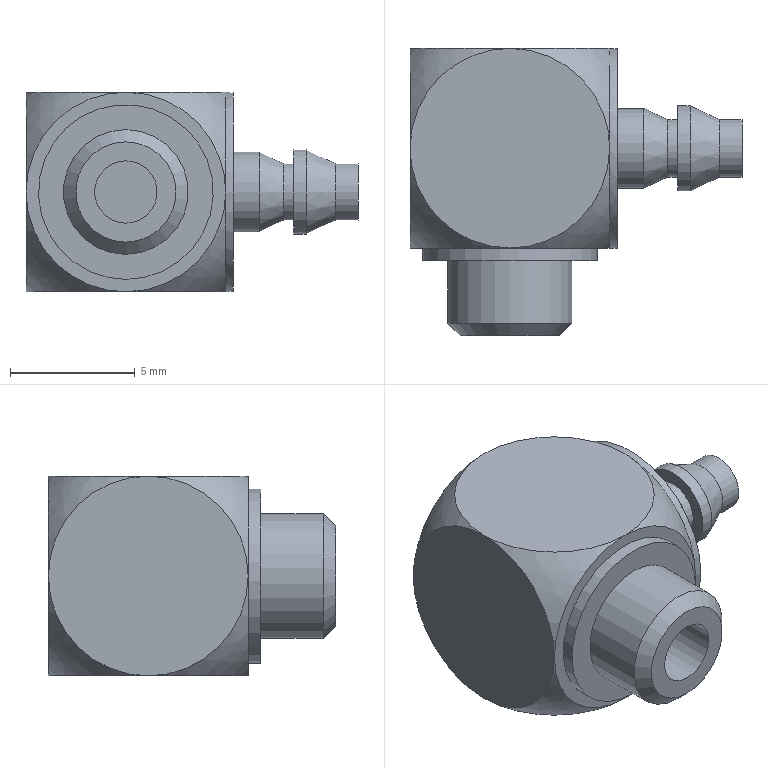Part | NX | 1 solid | 37 faces | box 13.3 x 11.5 x 8 mm | volume 560.169 mm3 | plane 15 | cylinder 11 | spline 8 | cone 3 | commonest cylinder face diameters 7 x3 2.3 x2 1.8 x1 2.5 x1 3.2 x1 3.4 x1
STEP:
#1=CARTESIAN_POINT('',(-4.,7.5,4.));
#2=VERTEX_POINT('',#1);
#3=CARTESIAN_POINT('',(0.,11.5,4.));
#4=VERTEX_POINT('',#3);
#5=CARTESIAN_POINT('',(-4.,7.5,4.));
#6=CARTESIAN_POINT('',(-4.,8.556,4.));
#7=CARTESIAN_POINT('',(-3.131,10.627,4.));
#8=CARTESIAN_POINT('',(-1.056,11.5,4.));
#9=CARTESIAN_POINT('',(0.,11.5,4.));
#10=B_SPLINE_CURVE_WITH_KNOTS('',3,(#5,#6,#7,#8,#9),.UNSPECIFIED.,.F.,.F.,(4,1,4),(0.,0.003124,0.006249),.UNSPECIFIED.);
#11=EDGE_CURVE('',#2,#4,#10,.T.);
#12=ORIENTED_EDGE('',*,*,#11,.F.);
#13=CARTESIAN_POINT('',(0.,3.5,4.));
#14=VERTEX_POINT('',#13);
#15=CARTESIAN_POINT('',(0.,3.5,4.));
#16=CARTESIAN_POINT('',(-1.056,3.5,4.));
#17=CARTESIAN_POINT('',(-3.127,4.369,4.));
#18=CARTESIAN_POINT('',(-4.,6.444,4.));
#19=CARTESIAN_POINT('',(-4.,7.5,4.));
#20=B_SPLINE_CURVE_WITH_KNOTS('',3,(#15,#16,#17,#18,#19),.UNSPECIFIED.,.F.,.F.,(4,1,4),(0.,0.003124,0.006249),.UNSPECIFIED.);
#21=EDGE_CURVE('',#14,#2,#20,.T.);
#22=ORIENTED_EDGE('',*,*,#21,.F.);
#23=CARTESIAN_POINT('',(4.,7.5,4.));
#24=VERTEX_POINT('',#23);
#25=CARTESIAN_POINT('',(4.,7.5,4.));
#26=CARTESIAN_POINT('',(4.,6.444,4.));
#27=CARTESIAN_POINT('',(3.131,4.373,4.));
#28=CARTESIAN_POINT('',(1.056,3.5,4.));
#29=CARTESIAN_POINT('',(0.,3.5,4.));
#30=B_SPLINE_CURVE_WITH_KNOTS('',3,(#25,#26,#27,#28,#29),.UNSPECIFIED.,.F.,.F.,(4,1,4),(0.,0.003124,0.006249),.UNSPECIFIED.);
#31=EDGE_CURVE('',#24,#14,#30,.T.);
#32=ORIENTED_EDGE('',*,*,#31,.F.);
#33=CARTESIAN_POINT('',(0.,11.5,4.));
#34=CARTESIAN_POINT('',(1.056,11.5,4.));
#35=CARTESIAN_POINT('',(3.127,10.631,4.));
#36=CARTESIAN_POINT('',(4.,8.556,4.));
#37=CARTESIAN_POINT('',(4.,7.5,4.));
#38=B_SPLINE_CURVE_WITH_KNOTS('',3,(#33,#34,#35,#36,#37),.UNSPECIFIED.,.F.,.F.,(4,1,4),(0.,0.003124,0.006249),.UNSPECIFIED.);
#39=EDGE_CURVE('',#4,#24,#38,.T.);
#40=ORIENTED_EDGE('',*,*,#39,.F.);
#41=EDGE_LOOP('',(#12,#22,#32,#40));
#42=FACE_BOUND('',#41,.T.);
#43=CARTESIAN_POINT('',(-4.,3.5,4.));
#44=DIRECTION('',(0.,0.,-1.));
#45=DIRECTION('',(-1.,0.,0.));
#46=AXIS2_PLACEMENT_3D('',#43,#44,#45);
#47=PLANE('',#46);
#48=ADVANCED_FACE('',(#42),#47,.F.);
#49=CARTESIAN_POINT('',(4.,11.5,0.));
#50=VERTEX_POINT('',#49);
#51=CARTESIAN_POINT('',(4.,11.5,0.));
#52=CARTESIAN_POINT('',(4.,11.5,1.056));
#53=CARTESIAN_POINT('',(3.131,11.5,3.127));
#54=CARTESIAN_POINT('',(1.056,11.5,4.));
#55=CARTESIAN_POINT('',(0.,11.5,4.));
#56=B_SPLINE_CURVE_WITH_KNOTS('',3,(#51,#52,#53,#54,#55),.UNSPECIFIED.,.F.,.F.,(4,1,4),(0.,0.003124,0.006249),.UNSPECIFIED.);
#57=EDGE_CURVE('',#50,#4,#56,.T.);
#58=ORIENTED_EDGE('',*,*,#57,.T.);
#59=ORIENTED_EDGE('',*,*,#39,.T.);
#60=CARTESIAN_POINT('',(4.,7.5,0.));
#61=DIRECTION('',(1.,0.,0.));
#62=DIRECTION('',(0.,1.,0.));
#63=AXIS2_PLACEMENT_3D('',#60,#61,#62);
#64=CIRCLE('',#63,4.);
#65=EDGE_CURVE('',#24,#50,#64,.F.);
#66=ORIENTED_EDGE('',*,*,#65,.T.);
#67=EDGE_LOOP('',(#58,#59,#66));
#68=FACE_BOUND('',#67,.T.);
#69=CARTESIAN_POINT('',(4.,11.5,0.));
#70=CARTESIAN_POINT('',(4.,11.5,2.361));
#71=CARTESIAN_POINT('',(4.,9.823,4.022));
#72=CARTESIAN_POINT('',(4.,7.462,4.));
#73=CARTESIAN_POINT('',(2.947,12.553,0.));
#74=CARTESIAN_POINT('',(2.947,12.553,2.982));
#75=CARTESIAN_POINT('',(2.947,10.435,5.081));
#76=CARTESIAN_POINT('',(2.947,7.452,5.053));
#77=CARTESIAN_POINT('',(1.463,13.164,0.));
#78=CARTESIAN_POINT('',(1.463,13.164,3.343));
#79=CARTESIAN_POINT('',(1.463,10.789,5.695));
#80=CARTESIAN_POINT('',(1.463,7.447,5.664));
#81=CARTESIAN_POINT('',(-0.02666,13.157,0.));
#82=CARTESIAN_POINT('',(-0.02666,13.157,3.338));
#83=CARTESIAN_POINT('',(-0.02666,10.785,5.688));
#84=CARTESIAN_POINT('',(-0.02666,7.447,5.657));
#85=(BOUNDED_SURFACE()B_SPLINE_SURFACE(3,3,((#69,#70,#71,#72),(#73,#74,#75,#76),(#77,#78,#79,#80),(#81,#82,#83,#84)),.SURF_OF_REVOLUTION.,.F.,.F.,.F.)B_SPLINE_SURFACE_WITH_KNOTS((4,4),(4,4),(0.7854,1.576),(0.,1.),.PIECEWISE_BEZIER_KNOTS.)GEOMETRIC_REPRESENTATION_ITEM()RATIONAL_B_SPLINE_SURFACE(((1.,0.8025,0.8025,1.),(1.,0.8025,0.8025,1.),(1.,0.8025,0.8025,1.),(1.,0.8025,0.8025,1.)))REPRESENTATION_ITEM('')SURFACE());
#86=ADVANCED_FACE('',(#68),#85,.T.);
#87=ORIENTED_EDGE('',*,*,#11,.T.);
#88=CARTESIAN_POINT('',(-4.,11.5,0.));
#89=VERTEX_POINT('',#88);
#90=CARTESIAN_POINT('',(0.,11.5,4.));
#91=CARTESIAN_POINT('',(-1.056,11.5,4.));
#92=CARTESIAN_POINT('',(-3.127,11.5,3.131));
#93=CARTESIAN_POINT('',(-4.,11.5,1.056));
#94=CARTESIAN_POINT('',(-4.,11.5,0.));
#95=B_SPLINE_CURVE_WITH_KNOTS('',3,(#90,#91,#92,#93,#94),.UNSPECIFIED.,.F.,.F.,(4,1,4),(0.,0.003124,0.006249),.UNSPECIFIED.);
#96=EDGE_CURVE('',#4,#89,#95,.T.);
#97=ORIENTED_EDGE('',*,*,#96,.T.);
#98=CARTESIAN_POINT('',(-4.,7.5,0.));
#99=DIRECTION('',(1.,0.,0.));
#100=DIRECTION('',(0.,0.,-1.));
#101=AXIS2_PLACEMENT_3D('',#98,#99,#100);
#102=CIRCLE('',#101,4.);
#103=EDGE_CURVE('',#89,#2,#102,.T.);
#104=ORIENTED_EDGE('',*,*,#103,.T.);
#105=EDGE_LOOP('',(#87,#97,#104));
#106=FACE_BOUND('',#105,.T.);
#107=CARTESIAN_POINT('',(0.02666,13.157,0.));
#108=CARTESIAN_POINT('',(0.02666,13.157,3.338));
#109=CARTESIAN_POINT('',(0.02666,10.785,5.688));
#110=CARTESIAN_POINT('',(0.02666,7.447,5.657));
#111=CARTESIAN_POINT('',(-1.463,13.164,0.));
#112=CARTESIAN_POINT('',(-1.463,13.164,3.343));
#113=CARTESIAN_POINT('',(-1.463,10.789,5.695));
#114=CARTESIAN_POINT('',(-1.463,7.447,5.664));
#115=CARTESIAN_POINT('',(-2.947,12.553,0.));
#116=CARTESIAN_POINT('',(-2.947,12.553,2.982));
#117=CARTESIAN_POINT('',(-2.947,10.435,5.081));
#118=CARTESIAN_POINT('',(-2.947,7.452,5.053));
#119=CARTESIAN_POINT('',(-4.,11.5,0.));
#120=CARTESIAN_POINT('',(-4.,11.5,2.361));
#121=CARTESIAN_POINT('',(-4.,9.823,4.022));
#122=CARTESIAN_POINT('',(-4.,7.462,4.));
#123=(BOUNDED_SURFACE()B_SPLINE_SURFACE(3,3,((#107,#108,#109,#110),(#111,#112,#113,#114),(#115,#116,#117,#118),(#119,#120,#121,#122)),.SURF_OF_REVOLUTION.,.F.,.F.,.F.)B_SPLINE_SURFACE_WITH_KNOTS((4,4),(4,4),(1.566,2.356),(0.,1.),.PIECEWISE_BEZIER_KNOTS.)GEOMETRIC_REPRESENTATION_ITEM()RATIONAL_B_SPLINE_SURFACE(((1.,0.8025,0.8025,1.),(1.,0.8025,0.8025,1.),(1.,0.8025,0.8025,1.),(1.,0.8025,0.8025,1.)))REPRESENTATION_ITEM('')SURFACE());
#124=ADVANCED_FACE('',(#106),#123,.T.);
#125=CARTESIAN_POINT('',(-4.,3.5,0.));
#126=VERTEX_POINT('',#125);
#127=CARTESIAN_POINT('',(-4.,3.5,0.));
#128=CARTESIAN_POINT('',(-4.,3.5,1.056));
#129=CARTESIAN_POINT('',(-3.131,3.5,3.127));
#130=CARTESIAN_POINT('',(-1.056,3.5,4.));
#131=CARTESIAN_POINT('',(0.,3.5,4.));
#132=B_SPLINE_CURVE_WITH_KNOTS('',3,(#127,#128,#129,#130,#131),.UNSPECIFIED.,.F.,.F.,(4,1,4),(0.,0.003124,0.006249),.UNSPECIFIED.);
#133=EDGE_CURVE('',#126,#14,#132,.T.);
#134=ORIENTED_EDGE('',*,*,#133,.T.);
#135=ORIENTED_EDGE('',*,*,#21,.T.);
#136=CARTESIAN_POINT('',(-4.,7.5,0.));
#137=DIRECTION('',(1.,0.,0.));
#138=DIRECTION('',(0.,0.,-1.));
#139=AXIS2_PLACEMENT_3D('',#136,#137,#138);
#140=CIRCLE('',#139,4.);
#141=EDGE_CURVE('',#2,#126,#140,.T.);
#142=ORIENTED_EDGE('',*,*,#141,.T.);
#143=EDGE_LOOP('',(#134,#135,#142));
#144=FACE_BOUND('',#143,.T.);
#145=CARTESIAN_POINT('',(0.02666,7.553,5.657));
#146=CARTESIAN_POINT('',(0.02666,4.19,5.688));
#147=CARTESIAN_POINT('',(0.02666,1.812,3.31));
#148=CARTESIAN_POINT('',(0.02666,1.843,-0.05331));
#149=CARTESIAN_POINT('',(-1.463,7.553,5.664));
#150=CARTESIAN_POINT('',(-1.463,4.186,5.695));
#151=CARTESIAN_POINT('',(-1.463,1.805,3.314));
#152=CARTESIAN_POINT('',(-1.463,1.836,-0.05338));
#153=CARTESIAN_POINT('',(-2.947,7.548,5.053));
#154=CARTESIAN_POINT('',(-2.947,4.543,5.082));
#155=CARTESIAN_POINT('',(-2.947,2.418,2.957));
#156=CARTESIAN_POINT('',(-2.947,2.447,-0.04763));
#157=CARTESIAN_POINT('',(-4.,7.538,4.));
#158=CARTESIAN_POINT('',(-4.,5.159,4.022));
#159=CARTESIAN_POINT('',(-4.,3.478,2.341));
#160=CARTESIAN_POINT('',(-4.,3.5,-0.0377));
#161=(BOUNDED_SURFACE()B_SPLINE_SURFACE(3,3,((#145,#146,#147,#148),(#149,#150,#151,#152),(#153,#154,#155,#156),(#157,#158,#159,#160)),.SURF_OF_REVOLUTION.,.F.,.F.,.F.)B_SPLINE_SURFACE_WITH_KNOTS((4,4),(4,4),(1.566,2.356),(0.,1.),.PIECEWISE_BEZIER_KNOTS.)GEOMETRIC_REPRESENTATION_ITEM()RATIONAL_B_SPLINE_SURFACE(((1.,0.8003,0.8003,1.),(1.,0.8003,0.8003,1.),(1.,0.8003,0.8003,1.),(1.,0.8003,0.8003,1.)))REPRESENTATION_ITEM('')SURFACE());
#162=ADVANCED_FACE('',(#144),#161,.T.);
#163=CARTESIAN_POINT('',(4.,3.5,0.));
#164=VERTEX_POINT('',#163);
#165=CARTESIAN_POINT('',(0.,3.5,4.));
#166=CARTESIAN_POINT('',(1.056,3.5,4.));
#167=CARTESIAN_POINT('',(3.127,3.5,3.131));
#168=CARTESIAN_POINT('',(4.,3.5,1.056));
#169=CARTESIAN_POINT('',(4.,3.5,0.));
#170=B_SPLINE_CURVE_WITH_KNOTS('',3,(#165,#166,#167,#168,#169),.UNSPECIFIED.,.F.,.F.,(4,1,4),(0.,0.003124,0.006249),.UNSPECIFIED.);
#171=EDGE_CURVE('',#14,#164,#170,.T.);
#172=ORIENTED_EDGE('',*,*,#171,.T.);
#173=CARTESIAN_POINT('',(4.,7.5,0.));
#174=DIRECTION('',(1.,0.,0.));
#175=DIRECTION('',(0.,1.,0.));
#176=AXIS2_PLACEMENT_3D('',#173,#174,#175);
#177=CIRCLE('',#176,4.);
#178=EDGE_CURVE('',#164,#24,#177,.F.);
#179=ORIENTED_EDGE('',*,*,#178,.T.);
#180=ORIENTED_EDGE('',*,*,#31,.T.);
#181=EDGE_LOOP('',(#172,#179,#180));
#182=FACE_BOUND('',#181,.T.);
#183=CARTESIAN_POINT('',(4.,7.538,4.));
#184=CARTESIAN_POINT('',(4.,5.159,4.022));
#185=CARTESIAN_POINT('',(4.,3.478,2.341));
#186=CARTESIAN_POINT('',(4.,3.5,-0.0377));
#187=CARTESIAN_POINT('',(2.947,7.548,5.053));
#188=CARTESIAN_POINT('',(2.947,4.543,5.082));
#189=CARTESIAN_POINT('',(2.947,2.418,2.957));
#190=CARTESIAN_POINT('',(2.947,2.447,-0.04763));
#191=CARTESIAN_POINT('',(1.463,7.553,5.664));
#192=CARTESIAN_POINT('',(1.463,4.186,5.695));
#193=CARTESIAN_POINT('',(1.463,1.805,3.314));
#194=CARTESIAN_POINT('',(1.463,1.836,-0.05338));
#195=CARTESIAN_POINT('',(-0.02666,7.553,5.657));
#196=CARTESIAN_POINT('',(-0.02666,4.19,5.688));
#197=CARTESIAN_POINT('',(-0.02666,1.812,3.31));
#198=CARTESIAN_POINT('',(-0.02666,1.843,-0.05331));
#199=(BOUNDED_SURFACE()B_SPLINE_SURFACE(3,3,((#183,#184,#185,#186),(#187,#188,#189,#190),(#191,#192,#193,#194),(#195,#196,#197,#198)),.SURF_OF_REVOLUTION.,.F.,.F.,.F.)B_SPLINE_SURFACE_WITH_KNOTS((4,4),(4,4),(0.7854,1.576),(0.,1.),.PIECEWISE_BEZIER_KNOTS.)GEOMETRIC_REPRESENTATION_ITEM()RATIONAL_B_SPLINE_SURFACE(((1.,0.8003,0.8003,1.),(1.,0.8003,0.8003,1.),(1.,0.8003,0.8003,1.),(1.,0.8003,0.8003,1.)))REPRESENTATION_ITEM('')SURFACE());
#200=ADVANCED_FACE('',(#182),#199,.T.);
#201=ORIENTED_EDGE('',*,*,#57,.F.);
#202=CARTESIAN_POINT('',(0.,11.5,-4.));
#203=VERTEX_POINT('',#202);
#204=CARTESIAN_POINT('',(4.,11.5,0.));
#205=CARTESIAN_POINT('',(4.,11.5,-1.056));
#206=CARTESIAN_POINT('',(3.131,11.5,-3.127));
#207=CARTESIAN_POINT('',(1.056,11.5,-4.));
#208=CARTESIAN_POINT('',(0.,11.5,-4.));
#209=B_SPLINE_CURVE_WITH_KNOTS('',3,(#204,#205,#206,#207,#208),.UNSPECIFIED.,.F.,.F.,(4,1,4),(0.,0.003124,0.006249),.UNSPECIFIED.);
#210=EDGE_CURVE('',#50,#203,#209,.T.);
#211=ORIENTED_EDGE('',*,*,#210,.T.);
#212=CARTESIAN_POINT('',(0.,11.5,-4.));
#213=CARTESIAN_POINT('',(-1.056,11.5,-4.));
#214=CARTESIAN_POINT('',(-3.127,11.5,-3.131));
#215=CARTESIAN_POINT('',(-4.,11.5,-1.056));
#216=CARTESIAN_POINT('',(-4.,11.5,0.));
#217=B_SPLINE_CURVE_WITH_KNOTS('',3,(#212,#213,#214,#215,#216),.UNSPECIFIED.,.F.,.F.,(4,1,4),(0.,0.003124,0.006249),.UNSPECIFIED.);
#218=EDGE_CURVE('',#203,#89,#217,.T.);
#219=ORIENTED_EDGE('',*,*,#218,.T.);
#220=ORIENTED_EDGE('',*,*,#96,.F.);
#221=EDGE_LOOP('',(#201,#211,#219,#220));
#222=FACE_BOUND('',#221,.T.);
#223=CARTESIAN_POINT('',(-0.6,11.5,3.448));
#224=VERTEX_POINT('',#223);
#225=CARTESIAN_POINT('',(-0.6,11.5,-3.448));
#226=VERTEX_POINT('',#225);
#227=CARTESIAN_POINT('',(-0.6,11.5,-2.));
#228=DIRECTION('',(0.,0.,1.));
#229=VECTOR('',#228,1000.);
#230=LINE('',#227,#229);
#231=EDGE_CURVE('',#224,#226,#230,.F.);
#232=ORIENTED_EDGE('',*,*,#231,.T.);
#233=CARTESIAN_POINT('',(0.6,11.5,-3.448));
#234=VERTEX_POINT('',#233);
#235=CARTESIAN_POINT('',(0.,11.5,0.));
#236=DIRECTION('',(0.,1.,0.));
#237=DIRECTION('',(0.,0.,1.));
#238=AXIS2_PLACEMENT_3D('',#235,#236,#237);
#239=CIRCLE('',#238,3.5);
#240=EDGE_CURVE('',#226,#234,#239,.F.);
#241=ORIENTED_EDGE('',*,*,#240,.T.);
#242=CARTESIAN_POINT('',(0.6,11.5,3.448));
#243=VERTEX_POINT('',#242);
#244=CARTESIAN_POINT('',(0.6,11.5,-2.));
#245=DIRECTION('',(0.,0.,1.));
#246=VECTOR('',#245,1000.);
#247=LINE('',#244,#246);
#248=EDGE_CURVE('',#234,#243,#247,.T.);
#249=ORIENTED_EDGE('',*,*,#248,.T.);
#250=CARTESIAN_POINT('',(0.,11.5,0.));
#251=DIRECTION('',(0.,1.,0.));
#252=DIRECTION('',(0.,0.,1.));
#253=AXIS2_PLACEMENT_3D('',#250,#251,#252);
#254=CIRCLE('',#253,3.5);
#255=EDGE_CURVE('',#243,#224,#254,.F.);
#256=ORIENTED_EDGE('',*,*,#255,.T.);
#257=EDGE_LOOP('',(#232,#241,#249,#256));
#258=FACE_BOUND('',#257,.T.);
#259=CARTESIAN_POINT('',(0.,11.5,-2.));
#260=DIRECTION('',(0.,1.,0.));
#261=DIRECTION('',(0.,0.,1.));
#262=AXIS2_PLACEMENT_3D('',#259,#260,#261);
#263=PLANE('',#262);
#264=ADVANCED_FACE('',(#222,#258),#263,.T.);
#265=CARTESIAN_POINT('',(4.3,11.5,0.));
#266=VERTEX_POINT('',#265);
#267=CARTESIAN_POINT('',(4.3,7.5,0.));
#268=DIRECTION('',(1.,0.,0.));
#269=DIRECTION('',(0.,1.,0.));
#270=AXIS2_PLACEMENT_3D('',#267,#268,#269);
#271=CIRCLE('',#270,4.);
#272=EDGE_CURVE('',#266,#266,#271,.F.);
#273=ORIENTED_EDGE('',*,*,#272,.T.);
#274=EDGE_LOOP('',(#273));
#275=FACE_BOUND('',#274,.T.);
#276=ORIENTED_EDGE('',*,*,#178,.F.);
#277=CARTESIAN_POINT('',(4.,7.5,-4.));
#278=VERTEX_POINT('',#277);
#279=CARTESIAN_POINT('',(4.,7.5,0.));
#280=DIRECTION('',(1.,0.,0.));
#281=DIRECTION('',(0.,1.,0.));
#282=AXIS2_PLACEMENT_3D('',#279,#280,#281);
#283=CIRCLE('',#282,4.);
#284=EDGE_CURVE('',#278,#164,#283,.F.);
#285=ORIENTED_EDGE('',*,*,#284,.F.);
#286=CARTESIAN_POINT('',(4.,7.5,0.));
#287=DIRECTION('',(1.,0.,0.));
#288=DIRECTION('',(0.,1.,0.));
#289=AXIS2_PLACEMENT_3D('',#286,#287,#288);
#290=CIRCLE('',#289,4.);
#291=EDGE_CURVE('',#50,#278,#290,.F.);
#292=ORIENTED_EDGE('',*,*,#291,.F.);
#293=ORIENTED_EDGE('',*,*,#65,.F.);
#294=EDGE_LOOP('',(#276,#285,#292,#293));
#295=FACE_BOUND('',#294,.T.);
#296=CARTESIAN_POINT('',(4.15,7.5,0.));
#297=DIRECTION('',(1.,0.,0.));
#298=DIRECTION('',(0.,1.,0.));
#299=AXIS2_PLACEMENT_3D('',#296,#297,#298);
#300=CYLINDRICAL_SURFACE('',#299,4.);
#301=ADVANCED_FACE('',(#275,#295),#300,.T.);
#302=ORIENTED_EDGE('',*,*,#103,.F.);
#303=CARTESIAN_POINT('',(-4.,7.5,-4.));
#304=VERTEX_POINT('',#303);
#305=CARTESIAN_POINT('',(-4.,7.5,0.));
#306=DIRECTION('',(1.,0.,0.));
#307=DIRECTION('',(0.,0.,-1.));
#308=AXIS2_PLACEMENT_3D('',#305,#306,#307);
#309=CIRCLE('',#308,4.);
#310=EDGE_CURVE('',#304,#89,#309,.T.);
#311=ORIENTED_EDGE('',*,*,#310,.F.);
#312=CARTESIAN_POINT('',(-4.,7.5,0.));
#313=DIRECTION('',(1.,0.,0.));
#314=DIRECTION('',(0.,0.,-1.));
#315=AXIS2_PLACEMENT_3D('',#312,#313,#314);
#316=CIRCLE('',#315,4.);
#317=EDGE_CURVE('',#126,#304,#316,.T.);
#318=ORIENTED_EDGE('',*,*,#317,.F.);
#319=ORIENTED_EDGE('',*,*,#141,.F.);
#320=EDGE_LOOP('',(#302,#311,#318,#319));
#321=FACE_BOUND('',#320,.T.);
#322=CARTESIAN_POINT('',(-4.,3.5,-4.));
#323=DIRECTION('',(1.,0.,0.));
#324=DIRECTION('',(0.,0.,-1.));
#325=AXIS2_PLACEMENT_3D('',#322,#323,#324);
#326=PLANE('',#325);
#327=ADVANCED_FACE('',(#321),#326,.F.);
#328=CARTESIAN_POINT('',(0.,3.5,-3.5));
#329=VERTEX_POINT('',#328);
#330=CARTESIAN_POINT('',(0.,3.5,0.));
#331=DIRECTION('',(0.,-1.,0.));
#332=DIRECTION('',(0.,0.,-1.));
#333=AXIS2_PLACEMENT_3D('',#330,#331,#332);
#334=CIRCLE('',#333,3.5);
#335=EDGE_CURVE('',#329,#329,#334,.F.);
#336=ORIENTED_EDGE('',*,*,#335,.T.);
#337=EDGE_LOOP('',(#336));
#338=FACE_BOUND('',#337,.T.);
#339=ORIENTED_EDGE('',*,*,#171,.F.);
#340=ORIENTED_EDGE('',*,*,#133,.F.);
#341=CARTESIAN_POINT('',(0.,3.5,-4.));
#342=VERTEX_POINT('',#341);
#343=CARTESIAN_POINT('',(-4.,3.5,0.));
#344=CARTESIAN_POINT('',(-4.,3.5,-1.056));
#345=CARTESIAN_POINT('',(-3.131,3.5,-3.127));
#346=CARTESIAN_POINT('',(-1.056,3.5,-4.));
#347=CARTESIAN_POINT('',(0.,3.5,-4.));
#348=B_SPLINE_CURVE_WITH_KNOTS('',3,(#343,#344,#345,#346,#347),.UNSPECIFIED.,.F.,.F.,(4,1,4),(0.,0.003124,0.006249),.UNSPECIFIED.);
#349=EDGE_CURVE('',#126,#342,#348,.T.);
#350=ORIENTED_EDGE('',*,*,#349,.T.);
#351=CARTESIAN_POINT('',(0.,3.5,-4.));
#352=CARTESIAN_POINT('',(1.056,3.5,-4.));
#353=CARTESIAN_POINT('',(3.127,3.5,-3.131));
#354=CARTESIAN_POINT('',(4.,3.5,-1.056));
#355=CARTESIAN_POINT('',(4.,3.5,0.));
#356=B_SPLINE_CURVE_WITH_KNOTS('',3,(#351,#352,#353,#354,#355),.UNSPECIFIED.,.F.,.F.,(4,1,4),(0.,0.003124,0.006249),.UNSPECIFIED.);
#357=EDGE_CURVE('',#342,#164,#356,.T.);
#358=ORIENTED_EDGE('',*,*,#357,.T.);
#359=EDGE_LOOP('',(#339,#340,#350,#358));
#360=FACE_BOUND('',#359,.T.);
#361=CARTESIAN_POINT('',(0.,3.5,-3.75));
#362=DIRECTION('',(0.,-1.,0.));
#363=DIRECTION('',(0.,0.,-1.));
#364=AXIS2_PLACEMENT_3D('',#361,#362,#363);
#365=PLANE('',#364);
#366=ADVANCED_FACE('',(#338,#360),#365,.T.);
#367=ORIENTED_EDGE('',*,*,#210,.F.);
#368=ORIENTED_EDGE('',*,*,#291,.T.);
#369=CARTESIAN_POINT('',(4.,7.5,-4.));
#370=CARTESIAN_POINT('',(4.,8.556,-4.));
#371=CARTESIAN_POINT('',(3.131,10.627,-4.));
#372=CARTESIAN_POINT('',(1.056,11.5,-4.));
#373=CARTESIAN_POINT('',(0.,11.5,-4.));
#374=B_SPLINE_CURVE_WITH_KNOTS('',3,(#369,#370,#371,#372,#373),.UNSPECIFIED.,.F.,.F.,(4,1,4),(0.,0.003124,0.006249),.UNSPECIFIED.);
#375=EDGE_CURVE('',#278,#203,#374,.T.);
#376=ORIENTED_EDGE('',*,*,#375,.T.);
#377=EDGE_LOOP('',(#367,#368,#376));
#378=FACE_BOUND('',#377,.T.);
#379=CARTESIAN_POINT('',(4.,7.462,-4.));
#380=CARTESIAN_POINT('',(4.,9.841,-4.022));
#381=CARTESIAN_POINT('',(4.,11.522,-2.341));
#382=CARTESIAN_POINT('',(4.,11.5,0.0377));
#383=CARTESIAN_POINT('',(2.947,7.452,-5.053));
#384=CARTESIAN_POINT('',(2.947,10.457,-5.082));
#385=CARTESIAN_POINT('',(2.947,12.582,-2.957));
#386=CARTESIAN_POINT('',(2.947,12.553,0.04763));
#387=CARTESIAN_POINT('',(1.463,7.447,-5.664));
#388=CARTESIAN_POINT('',(1.463,10.814,-5.695));
#389=CARTESIAN_POINT('',(1.463,13.195,-3.314));
#390=CARTESIAN_POINT('',(1.463,13.164,0.05338));
#391=CARTESIAN_POINT('',(-0.02666,7.447,-5.657));
#392=CARTESIAN_POINT('',(-0.02666,10.81,-5.688));
#393=CARTESIAN_POINT('',(-0.02666,13.188,-3.31));
#394=CARTESIAN_POINT('',(-0.02666,13.157,0.05331));
#395=(BOUNDED_SURFACE()B_SPLINE_SURFACE(3,3,((#379,#380,#381,#382),(#383,#384,#385,#386),(#387,#388,#389,#390),(#391,#392,#393,#394)),.SURF_OF_REVOLUTION.,.F.,.F.,.F.)B_SPLINE_SURFACE_WITH_KNOTS((4,4),(4,4),(0.7854,1.576),(0.,1.),.PIECEWISE_BEZIER_KNOTS.)GEOMETRIC_REPRESENTATION_ITEM()RATIONAL_B_SPLINE_SURFACE(((1.,0.8003,0.8003,1.),(1.,0.8003,0.8003,1.),(1.,0.8003,0.8003,1.),(1.,0.8003,0.8003,1.)))REPRESENTATION_ITEM('')SURFACE());
#396=ADVANCED_FACE('',(#378),#395,.T.);
#397=ORIENTED_EDGE('',*,*,#310,.T.);
#398=ORIENTED_EDGE('',*,*,#218,.F.);
#399=CARTESIAN_POINT('',(0.,11.5,-4.));
#400=CARTESIAN_POINT('',(-1.056,11.5,-4.));
#401=CARTESIAN_POINT('',(-3.127,10.631,-4.));
#402=CARTESIAN_POINT('',(-4.,8.556,-4.));
#403=CARTESIAN_POINT('',(-4.,7.5,-4.));
#404=B_SPLINE_CURVE_WITH_KNOTS('',3,(#399,#400,#401,#402,#403),.UNSPECIFIED.,.F.,.F.,(4,1,4),(0.,0.003124,0.006249),.UNSPECIFIED.);
#405=EDGE_CURVE('',#203,#304,#404,.T.);
#406=ORIENTED_EDGE('',*,*,#405,.T.);
#407=EDGE_LOOP('',(#397,#398,#406));
#408=FACE_BOUND('',#407,.T.);
#409=CARTESIAN_POINT('',(0.02666,7.447,-5.657));
#410=CARTESIAN_POINT('',(0.02666,10.81,-5.688));
#411=CARTESIAN_POINT('',(0.02666,13.188,-3.31));
#412=CARTESIAN_POINT('',(0.02666,13.157,0.05331));
#413=CARTESIAN_POINT('',(-1.463,7.447,-5.664));
#414=CARTESIAN_POINT('',(-1.463,10.814,-5.695));
#415=CARTESIAN_POINT('',(-1.463,13.195,-3.314));
#416=CARTESIAN_POINT('',(-1.463,13.164,0.05338));
#417=CARTESIAN_POINT('',(-2.947,7.452,-5.053));
#418=CARTESIAN_POINT('',(-2.947,10.457,-5.082));
#419=CARTESIAN_POINT('',(-2.947,12.582,-2.957));
#420=CARTESIAN_POINT('',(-2.947,12.553,0.04763));
#421=CARTESIAN_POINT('',(-4.,7.462,-4.));
#422=CARTESIAN_POINT('',(-4.,9.841,-4.022));
#423=CARTESIAN_POINT('',(-4.,11.522,-2.341));
#424=CARTESIAN_POINT('',(-4.,11.5,0.0377));
#425=(BOUNDED_SURFACE()B_SPLINE_SURFACE(3,3,((#409,#410,#411,#412),(#413,#414,#415,#416),(#417,#418,#419,#420),(#421,#422,#423,#424)),.SURF_OF_REVOLUTION.,.F.,.F.,.F.)B_SPLINE_SURFACE_WITH_KNOTS((4,4),(4,4),(1.566,2.356),(0.,1.),.PIECEWISE_BEZIER_KNOTS.)GEOMETRIC_REPRESENTATION_ITEM()RATIONAL_B_SPLINE_SURFACE(((1.,0.8003,0.8003,1.),(1.,0.8003,0.8003,1.),(1.,0.8003,0.8003,1.),(1.,0.8003,0.8003,1.)))REPRESENTATION_ITEM('')SURFACE());
#426=ADVANCED_FACE('',(#408),#425,.T.);
#427=CARTESIAN_POINT('',(0.6,10.,-3.448));
#428=VERTEX_POINT('',#427);
#429=CARTESIAN_POINT('',(0.6,11.5,-3.448));
#430=DIRECTION('',(0.,1.,0.));
#431=VECTOR('',#430,1000.);
#432=LINE('',#429,#431);
#433=EDGE_CURVE('',#234,#428,#432,.F.);
#434=ORIENTED_EDGE('',*,*,#433,.F.);
#435=ORIENTED_EDGE('',*,*,#240,.F.);
#436=CARTESIAN_POINT('',(-0.6,10.,-3.448));
#437=VERTEX_POINT('',#436);
#438=CARTESIAN_POINT('',(-0.6,11.5,-3.448));
#439=DIRECTION('',(0.,1.,0.));
#440=VECTOR('',#439,1000.);
#441=LINE('',#438,#440);
#442=EDGE_CURVE('',#437,#226,#441,.T.);
#443=ORIENTED_EDGE('',*,*,#442,.F.);
#444=CARTESIAN_POINT('',(0.,10.,0.));
#445=DIRECTION('',(0.,1.,0.));
#446=DIRECTION('',(0.,0.,1.));
#447=AXIS2_PLACEMENT_3D('',#444,#445,#446);
#448=CIRCLE('',#447,3.5);
#449=EDGE_CURVE('',#428,#437,#448,.T.);
#450=ORIENTED_EDGE('',*,*,#449,.F.);
#451=EDGE_LOOP('',(#434,#435,#443,#450));
#452=FACE_BOUND('',#451,.T.);
#453=CARTESIAN_POINT('',(0.,11.5,0.));
#454=DIRECTION('',(0.,1.,0.));
#455=DIRECTION('',(0.,0.,1.));
#456=AXIS2_PLACEMENT_3D('',#453,#454,#455);
#457=CYLINDRICAL_SURFACE('',#456,3.5);
#458=ADVANCED_FACE('',(#452),#457,.F.);
#459=ORIENTED_EDGE('',*,*,#442,.T.);
#460=ORIENTED_EDGE('',*,*,#231,.F.);
#461=CARTESIAN_POINT('',(-0.6,10.,3.448));
#462=VERTEX_POINT('',#461);
#463=CARTESIAN_POINT('',(-0.6,11.5,3.448));
#464=DIRECTION('',(0.,1.,0.));
#465=VECTOR('',#464,1000.);
#466=LINE('',#463,#465);
#467=EDGE_CURVE('',#462,#224,#466,.T.);
#468=ORIENTED_EDGE('',*,*,#467,.F.);
#469=CARTESIAN_POINT('',(-0.6,10.,-3.448));
#470=DIRECTION('',(0.,0.,1.));
#471=VECTOR('',#470,1000.);
#472=LINE('',#469,#471);
#473=EDGE_CURVE('',#437,#462,#472,.T.);
#474=ORIENTED_EDGE('',*,*,#473,.F.);
#475=EDGE_LOOP('',(#459,#460,#468,#474));
#476=FACE_BOUND('',#475,.T.);
#477=CARTESIAN_POINT('',(-0.6,11.5,-3.448));
#478=DIRECTION('',(-1.,0.,0.));
#479=DIRECTION('',(0.,0.,1.));
#480=AXIS2_PLACEMENT_3D('',#477,#478,#479);
#481=PLANE('',#480);
#482=ADVANCED_FACE('',(#476),#481,.F.);
#483=ORIENTED_EDGE('',*,*,#467,.T.);
#484=ORIENTED_EDGE('',*,*,#255,.F.);
#485=CARTESIAN_POINT('',(0.6,10.,3.448));
#486=VERTEX_POINT('',#485);
#487=CARTESIAN_POINT('',(0.6,11.5,3.448));
#488=DIRECTION('',(0.,1.,0.));
#489=VECTOR('',#488,1000.);
#490=LINE('',#487,#489);
#491=EDGE_CURVE('',#486,#243,#490,.T.);
#492=ORIENTED_EDGE('',*,*,#491,.F.);
#493=CARTESIAN_POINT('',(0.,10.,0.));
#494=DIRECTION('',(0.,1.,0.));
#495=DIRECTION('',(0.,0.,1.));
#496=AXIS2_PLACEMENT_3D('',#493,#494,#495);
#497=CIRCLE('',#496,3.5);
#498=EDGE_CURVE('',#462,#486,#497,.T.);
#499=ORIENTED_EDGE('',*,*,#498,.F.);
#500=EDGE_LOOP('',(#483,#484,#492,#499));
#501=FACE_BOUND('',#500,.T.);
#502=CARTESIAN_POINT('',(0.,11.5,0.));
#503=DIRECTION('',(0.,1.,0.));
#504=DIRECTION('',(0.,0.,1.));
#505=AXIS2_PLACEMENT_3D('',#502,#503,#504);
#506=CYLINDRICAL_SURFACE('',#505,3.5);
#507=ADVANCED_FACE('',(#501),#506,.F.);
#508=ORIENTED_EDGE('',*,*,#491,.T.);
#509=ORIENTED_EDGE('',*,*,#248,.F.);
#510=ORIENTED_EDGE('',*,*,#433,.T.);
#511=CARTESIAN_POINT('',(0.6,10.,3.448));
#512=DIRECTION('',(0.,0.,-1.));
#513=VECTOR('',#512,1000.);
#514=LINE('',#511,#513);
#515=EDGE_CURVE('',#486,#428,#514,.T.);
#516=ORIENTED_EDGE('',*,*,#515,.F.);
#517=EDGE_LOOP('',(#508,#509,#510,#516));
#518=FACE_BOUND('',#517,.T.);
#519=CARTESIAN_POINT('',(0.6,11.5,3.448));
#520=DIRECTION('',(1.,0.,0.));
#521=DIRECTION('',(0.,0.,-1.));
#522=AXIS2_PLACEMENT_3D('',#519,#520,#521);
#523=PLANE('',#522);
#524=ADVANCED_FACE('',(#518),#523,.F.);
#525=CARTESIAN_POINT('',(4.3,9.1,0.));
#526=VERTEX_POINT('',#525);
#527=CARTESIAN_POINT('',(4.3,7.5,0.));
#528=DIRECTION('',(1.,0.,0.));
#529=DIRECTION('',(0.,1.,0.));
#530=AXIS2_PLACEMENT_3D('',#527,#528,#529);
#531=CIRCLE('',#530,1.6);
#532=EDGE_CURVE('',#526,#526,#531,.F.);
#533=ORIENTED_EDGE('',*,*,#532,.T.);
#534=EDGE_LOOP('',(#533));
#535=FACE_BOUND('',#534,.T.);
#536=ORIENTED_EDGE('',*,*,#272,.F.);
#537=EDGE_LOOP('',(#536));
#538=FACE_BOUND('',#537,.T.);
#539=CARTESIAN_POINT('',(4.3,10.3,0.));
#540=DIRECTION('',(1.,0.,0.));
#541=DIRECTION('',(0.,0.,-1.));
#542=AXIS2_PLACEMENT_3D('',#539,#540,#541);
#543=PLANE('',#542);
#544=ADVANCED_FACE('',(#535,#538),#543,.T.);
#545=ORIENTED_EDGE('',*,*,#349,.F.);
#546=ORIENTED_EDGE('',*,*,#317,.T.);
#547=CARTESIAN_POINT('',(-4.,7.5,-4.));
#548=CARTESIAN_POINT('',(-4.,6.444,-4.));
#549=CARTESIAN_POINT('',(-3.131,4.373,-4.));
#550=CARTESIAN_POINT('',(-1.056,3.5,-4.));
#551=CARTESIAN_POINT('',(0.,3.5,-4.));
#552=B_SPLINE_CURVE_WITH_KNOTS('',3,(#547,#548,#549,#550,#551),.UNSPECIFIED.,.F.,.F.,(4,1,4),(0.,0.003124,0.006249),.UNSPECIFIED.);
#553=EDGE_CURVE('',#304,#342,#552,.T.);
#554=ORIENTED_EDGE('',*,*,#553,.T.);
#555=EDGE_LOOP('',(#545,#546,#554));
#556=FACE_BOUND('',#555,.T.);
#557=CARTESIAN_POINT('',(0.02666,1.843,0.05331));
#558=CARTESIAN_POINT('',(0.02666,1.812,-3.31));
#559=CARTESIAN_POINT('',(0.02666,4.19,-5.688));
#560=CARTESIAN_POINT('',(0.02666,7.553,-5.657));
#561=CARTESIAN_POINT('',(-1.463,1.836,0.05338));
#562=CARTESIAN_POINT('',(-1.463,1.805,-3.314));
#563=CARTESIAN_POINT('',(-1.463,4.186,-5.695));
#564=CARTESIAN_POINT('',(-1.463,7.553,-5.664));
#565=CARTESIAN_POINT('',(-2.947,2.447,0.04763));
#566=CARTESIAN_POINT('',(-2.947,2.418,-2.957));
#567=CARTESIAN_POINT('',(-2.947,4.543,-5.082));
#568=CARTESIAN_POINT('',(-2.947,7.548,-5.053));
#569=CARTESIAN_POINT('',(-4.,3.5,0.0377));
#570=CARTESIAN_POINT('',(-4.,3.478,-2.341));
#571=CARTESIAN_POINT('',(-4.,5.159,-4.022));
#572=CARTESIAN_POINT('',(-4.,7.538,-4.));
#573=(BOUNDED_SURFACE()B_SPLINE_SURFACE(3,3,((#557,#558,#559,#560),(#561,#562,#563,#564),(#565,#566,#567,#568),(#569,#570,#571,#572)),.SURF_OF_REVOLUTION.,.F.,.F.,.F.)B_SPLINE_SURFACE_WITH_KNOTS((4,4),(4,4),(1.566,2.356),(0.,1.),.PIECEWISE_BEZIER_KNOTS.)GEOMETRIC_REPRESENTATION_ITEM()RATIONAL_B_SPLINE_SURFACE(((1.,0.8003,0.8003,1.),(1.,0.8003,0.8003,1.),(1.,0.8003,0.8003,1.),(1.,0.8003,0.8003,1.)))REPRESENTATION_ITEM('')SURFACE());
#574=ADVANCED_FACE('',(#556),#573,.T.);
#575=ORIENTED_EDGE('',*,*,#335,.F.);
#576=EDGE_LOOP('',(#575));
#577=FACE_BOUND('',#576,.T.);
#578=CARTESIAN_POINT('',(0.,3.,-3.5));
#579=VERTEX_POINT('',#578);
#580=CARTESIAN_POINT('',(0.,3.,0.));
#581=DIRECTION('',(0.,-1.,0.));
#582=DIRECTION('',(0.,0.,-1.));
#583=AXIS2_PLACEMENT_3D('',#580,#581,#582);
#584=CIRCLE('',#583,3.5);
#585=EDGE_CURVE('',#579,#579,#584,.F.);
#586=ORIENTED_EDGE('',*,*,#585,.T.);
#587=EDGE_LOOP('',(#586));
#588=FACE_BOUND('',#587,.T.);
#589=CARTESIAN_POINT('',(0.,3.25,0.));
#590=DIRECTION('',(0.,-1.,0.));
#591=DIRECTION('',(0.,0.,-1.));
#592=AXIS2_PLACEMENT_3D('',#589,#590,#591);
#593=CYLINDRICAL_SURFACE('',#592,3.5);
#594=ADVANCED_FACE('',(#577,#588),#593,.T.);
#595=ORIENTED_EDGE('',*,*,#284,.T.);
#596=ORIENTED_EDGE('',*,*,#357,.F.);
#597=CARTESIAN_POINT('',(0.,3.5,-4.));
#598=CARTESIAN_POINT('',(1.056,3.5,-4.));
#599=CARTESIAN_POINT('',(3.127,4.369,-4.));
#600=CARTESIAN_POINT('',(4.,6.444,-4.));
#601=CARTESIAN_POINT('',(4.,7.5,-4.));
#602=B_SPLINE_CURVE_WITH_KNOTS('',3,(#597,#598,#599,#600,#601),.UNSPECIFIED.,.F.,.F.,(4,1,4),(0.,0.003124,0.006249),.UNSPECIFIED.);
#603=EDGE_CURVE('',#342,#278,#602,.T.);
#604=ORIENTED_EDGE('',*,*,#603,.T.);
#605=EDGE_LOOP('',(#595,#596,#604));
#606=FACE_BOUND('',#605,.T.);
#607=CARTESIAN_POINT('',(4.,3.5,0.0377));
#608=CARTESIAN_POINT('',(4.,3.478,-2.341));
#609=CARTESIAN_POINT('',(4.,5.159,-4.022));
#610=CARTESIAN_POINT('',(4.,7.538,-4.));
#611=CARTESIAN_POINT('',(2.947,2.447,0.04763));
#612=CARTESIAN_POINT('',(2.947,2.418,-2.957));
#613=CARTESIAN_POINT('',(2.947,4.543,-5.082));
#614=CARTESIAN_POINT('',(2.947,7.548,-5.053));
#615=CARTESIAN_POINT('',(1.463,1.836,0.05338));
#616=CARTESIAN_POINT('',(1.463,1.805,-3.314));
#617=CARTESIAN_POINT('',(1.463,4.186,-5.695));
#618=CARTESIAN_POINT('',(1.463,7.553,-5.664));
#619=CARTESIAN_POINT('',(-0.02666,1.843,0.05331));
#620=CARTESIAN_POINT('',(-0.02666,1.812,-3.31));
#621=CARTESIAN_POINT('',(-0.02666,4.19,-5.688));
#622=CARTESIAN_POINT('',(-0.02666,7.553,-5.657));
#623=(BOUNDED_SURFACE()B_SPLINE_SURFACE(3,3,((#607,#608,#609,#610),(#611,#612,#613,#614),(#615,#616,#617,#618),(#619,#620,#621,#622)),.SURF_OF_REVOLUTION.,.F.,.F.,.F.)B_SPLINE_SURFACE_WITH_KNOTS((4,4),(4,4),(0.7854,1.576),(0.,1.),.PIECEWISE_BEZIER_KNOTS.)GEOMETRIC_REPRESENTATION_ITEM()RATIONAL_B_SPLINE_SURFACE(((1.,0.8003,0.8003,1.),(1.,0.8003,0.8003,1.),(1.,0.8003,0.8003,1.),(1.,0.8003,0.8003,1.)))REPRESENTATION_ITEM('')SURFACE());
#624=ADVANCED_FACE('',(#606),#623,.T.);
#625=ORIENTED_EDGE('',*,*,#603,.F.);
#626=ORIENTED_EDGE('',*,*,#553,.F.);
#627=ORIENTED_EDGE('',*,*,#405,.F.);
#628=ORIENTED_EDGE('',*,*,#375,.F.);
#629=EDGE_LOOP('',(#625,#626,#627,#628));
#630=FACE_BOUND('',#629,.T.);
#631=CARTESIAN_POINT('',(4.,3.5,-4.));
#632=DIRECTION('',(0.,0.,1.));
#633=DIRECTION('',(1.,0.,0.));
#634=AXIS2_PLACEMENT_3D('',#631,#632,#633);
#635=PLANE('',#634);
#636=ADVANCED_FACE('',(#630),#635,.F.);
#637=ORIENTED_EDGE('',*,*,#473,.T.);
#638=ORIENTED_EDGE('',*,*,#498,.T.);
#639=ORIENTED_EDGE('',*,*,#515,.T.);
#640=ORIENTED_EDGE('',*,*,#449,.T.);
#641=EDGE_LOOP('',(#637,#638,#639,#640));
#642=FACE_BOUND('',#641,.T.);
#643=CARTESIAN_POINT('',(0.,10.,0.));
#644=DIRECTION('',(0.,1.,0.));
#645=DIRECTION('',(0.,0.,1.));
#646=AXIS2_PLACEMENT_3D('',#643,#644,#645);
#647=PLANE('',#646);
#648=ADVANCED_FACE('',(#642),#647,.T.);
#649=ORIENTED_EDGE('',*,*,#532,.F.);
#650=EDGE_LOOP('',(#649));
#651=FACE_BOUND('',#650,.T.);
#652=CARTESIAN_POINT('',(5.355,9.1,0.));
#653=VERTEX_POINT('',#652);
#654=CARTESIAN_POINT('',(5.355,7.5,0.));
#655=DIRECTION('',(1.,0.,0.));
#656=DIRECTION('',(0.,1.,0.));
#657=AXIS2_PLACEMENT_3D('',#654,#655,#656);
#658=CIRCLE('',#657,1.6);
#659=EDGE_CURVE('',#653,#653,#658,.F.);
#660=ORIENTED_EDGE('',*,*,#659,.T.);
#661=EDGE_LOOP('',(#660));
#662=FACE_BOUND('',#661,.T.);
#663=CARTESIAN_POINT('',(4.828,7.5,0.));
#664=DIRECTION('',(1.,0.,0.));
#665=DIRECTION('',(0.,1.,0.));
#666=AXIS2_PLACEMENT_3D('',#663,#664,#665);
#667=CYLINDRICAL_SURFACE('',#666,1.6);
#668=ADVANCED_FACE('',(#651,#662),#667,.T.);
#669=CARTESIAN_POINT('',(0.,3.,-2.5));
#670=VERTEX_POINT('',#669);
#671=CARTESIAN_POINT('',(0.,3.,0.));
#672=DIRECTION('',(0.,-1.,0.));
#673=DIRECTION('',(0.,0.,-1.));
#674=AXIS2_PLACEMENT_3D('',#671,#672,#673);
#675=CIRCLE('',#674,2.5);
#676=EDGE_CURVE('',#670,#670,#675,.F.);
#677=ORIENTED_EDGE('',*,*,#676,.T.);
#678=EDGE_LOOP('',(#677));
#679=FACE_BOUND('',#678,.T.);
#680=ORIENTED_EDGE('',*,*,#585,.F.);
#681=EDGE_LOOP('',(#680));
#682=FACE_BOUND('',#681,.T.);
#683=CARTESIAN_POINT('',(0.,3.,-3.));
#684=DIRECTION('',(0.,-1.,0.));
#685=DIRECTION('',(0.,0.,-1.));
#686=AXIS2_PLACEMENT_3D('',#683,#684,#685);
#687=PLANE('',#686);
#688=ADVANCED_FACE('',(#679,#682),#687,.T.);
#689=ORIENTED_EDGE('',*,*,#659,.F.);
#690=EDGE_LOOP('',(#689));
#691=FACE_BOUND('',#690,.T.);
#692=CARTESIAN_POINT('',(6.321,8.65,0.));
#693=VERTEX_POINT('',#692);
#694=CARTESIAN_POINT('',(6.321,7.5,0.));
#695=DIRECTION('',(-1.,0.,0.));
#696=DIRECTION('',(0.,1.,0.));
#697=AXIS2_PLACEMENT_3D('',#694,#695,#696);
#698=CIRCLE('',#697,1.15);
#699=EDGE_CURVE('',#693,#693,#698,.T.);
#700=ORIENTED_EDGE('',*,*,#699,.T.);
#701=EDGE_LOOP('',(#700));
#702=FACE_BOUND('',#701,.T.);
#703=CARTESIAN_POINT('',(5.355,7.5,0.));
#704=DIRECTION('',(-1.,0.,0.));
#705=DIRECTION('',(0.,-1.,0.));
#706=AXIS2_PLACEMENT_3D('',#703,#704,#705);
#707=CONICAL_SURFACE('',#706,1.6,0.4363);
#708=ADVANCED_FACE('',(#691,#702),#707,.T.);
#709=ORIENTED_EDGE('',*,*,#676,.F.);
#710=EDGE_LOOP('',(#709));
#711=FACE_BOUND('',#710,.T.);
#712=CARTESIAN_POINT('',(0.,0.4905,-2.5));
#713=VERTEX_POINT('',#712);
#714=CARTESIAN_POINT('',(0.,0.4905,0.));
#715=DIRECTION('',(0.,-1.,0.));
#716=DIRECTION('',(0.,0.,-1.));
#717=AXIS2_PLACEMENT_3D('',#714,#715,#716);
#718=CIRCLE('',#717,2.5);
#719=EDGE_CURVE('',#713,#713,#718,.F.);
#720=ORIENTED_EDGE('',*,*,#719,.T.);
#721=EDGE_LOOP('',(#720));
#722=FACE_BOUND('',#721,.T.);
#723=CARTESIAN_POINT('',(0.,1.745,0.));
#724=DIRECTION('',(0.,-1.,0.));
#725=DIRECTION('',(0.,0.,-1.));
#726=AXIS2_PLACEMENT_3D('',#723,#724,#725);
#727=CYLINDRICAL_SURFACE('',#726,2.5);
#728=ADVANCED_FACE('',(#711,#722),#727,.T.);
#729=ORIENTED_EDGE('',*,*,#699,.F.);
#730=EDGE_LOOP('',(#729));
#731=FACE_BOUND('',#730,.T.);
#732=CARTESIAN_POINT('',(6.721,8.65,0.));
#733=VERTEX_POINT('',#732);
#734=CARTESIAN_POINT('',(6.721,7.5,0.));
#735=DIRECTION('',(1.,0.,0.));
#736=DIRECTION('',(0.,1.,0.));
#737=AXIS2_PLACEMENT_3D('',#734,#735,#736);
#738=CIRCLE('',#737,1.15);
#739=EDGE_CURVE('',#733,#733,#738,.F.);
#740=ORIENTED_EDGE('',*,*,#739,.T.);
#741=EDGE_LOOP('',(#740));
#742=FACE_BOUND('',#741,.T.);
#743=CARTESIAN_POINT('',(6.521,7.5,0.));
#744=DIRECTION('',(1.,0.,0.));
#745=DIRECTION('',(0.,1.,0.));
#746=AXIS2_PLACEMENT_3D('',#743,#744,#745);
#747=CYLINDRICAL_SURFACE('',#746,1.15);
#748=ADVANCED_FACE('',(#731,#742),#747,.T.);
#749=ORIENTED_EDGE('',*,*,#719,.F.);
#750=EDGE_LOOP('',(#749));
#751=FACE_BOUND('',#750,.T.);
#752=CARTESIAN_POINT('',(0.,0.,2.01));
#753=VERTEX_POINT('',#752);
#754=CARTESIAN_POINT('',(0.,0.,0.));
#755=DIRECTION('',(0.,1.,0.));
#756=DIRECTION('',(0.,0.,1.));
#757=AXIS2_PLACEMENT_3D('',#754,#755,#756);
#758=CIRCLE('',#757,2.01);
#759=EDGE_CURVE('',#753,#753,#758,.T.);
#760=ORIENTED_EDGE('',*,*,#759,.T.);
#761=EDGE_LOOP('',(#760));
#762=FACE_BOUND('',#761,.T.);
#763=CARTESIAN_POINT('',(0.,0.4905,0.));
#764=DIRECTION('',(0.,1.,0.));
#765=DIRECTION('',(0.,0.,1.));
#766=AXIS2_PLACEMENT_3D('',#763,#764,#765);
#767=CONICAL_SURFACE('',#766,2.5,0.7854);
#768=ADVANCED_FACE('',(#751,#762),#767,.T.);
#769=CARTESIAN_POINT('',(6.721,9.2,0.));
#770=VERTEX_POINT('',#769);
#771=CARTESIAN_POINT('',(6.721,7.5,0.));
#772=DIRECTION('',(1.,0.,0.));
#773=DIRECTION('',(0.,1.,0.));
#774=AXIS2_PLACEMENT_3D('',#771,#772,#773);
#775=CIRCLE('',#774,1.7);
#776=EDGE_CURVE('',#770,#770,#775,.F.);
#777=ORIENTED_EDGE('',*,*,#776,.T.);
#778=EDGE_LOOP('',(#777));
#779=FACE_BOUND('',#778,.T.);
#780=ORIENTED_EDGE('',*,*,#739,.F.);
#781=EDGE_LOOP('',(#780));
#782=FACE_BOUND('',#781,.T.);
#783=CARTESIAN_POINT('',(6.721,8.925,0.));
#784=DIRECTION('',(-1.,0.,0.));
#785=DIRECTION('',(0.,0.,1.));
#786=AXIS2_PLACEMENT_3D('',#783,#784,#785);
#787=PLANE('',#786);
#788=ADVANCED_FACE('',(#779,#782),#787,.T.);
#789=ORIENTED_EDGE('',*,*,#759,.F.);
#790=EDGE_LOOP('',(#789));
#791=FACE_BOUND('',#790,.T.);
#792=CARTESIAN_POINT('',(0.,0.,-1.25));
#793=VERTEX_POINT('',#792);
#794=CARTESIAN_POINT('',(0.,0.,0.));
#795=DIRECTION('',(0.,-1.,0.));
#796=DIRECTION('',(0.,0.,-1.));
#797=AXIS2_PLACEMENT_3D('',#794,#795,#796);
#798=CIRCLE('',#797,1.25);
#799=EDGE_CURVE('',#793,#793,#798,.F.);
#800=ORIENTED_EDGE('',*,*,#799,.T.);
#801=EDGE_LOOP('',(#800));
#802=FACE_BOUND('',#801,.T.);
#803=CARTESIAN_POINT('',(0.,0.,-1.005));
#804=DIRECTION('',(0.,-1.,0.));
#805=DIRECTION('',(0.,0.,-1.));
#806=AXIS2_PLACEMENT_3D('',#803,#804,#805);
#807=PLANE('',#806);
#808=ADVANCED_FACE('',(#791,#802),#807,.T.);
#809=ORIENTED_EDGE('',*,*,#776,.F.);
#810=EDGE_LOOP('',(#809));
#811=FACE_BOUND('',#810,.T.);
#812=CARTESIAN_POINT('',(7.221,9.2,0.));
#813=VERTEX_POINT('',#812);
#814=CARTESIAN_POINT('',(7.221,7.5,0.));
#815=DIRECTION('',(1.,0.,0.));
#816=DIRECTION('',(0.,1.,0.));
#817=AXIS2_PLACEMENT_3D('',#814,#815,#816);
#818=CIRCLE('',#817,1.7);
#819=EDGE_CURVE('',#813,#813,#818,.F.);
#820=ORIENTED_EDGE('',*,*,#819,.T.);
#821=EDGE_LOOP('',(#820));
#822=FACE_BOUND('',#821,.T.);
#823=CARTESIAN_POINT('',(6.971,7.5,0.));
#824=DIRECTION('',(1.,0.,0.));
#825=DIRECTION('',(0.,1.,0.));
#826=AXIS2_PLACEMENT_3D('',#823,#824,#825);
#827=CYLINDRICAL_SURFACE('',#826,1.7);
#828=ADVANCED_FACE('',(#811,#822),#827,.T.);
#829=ORIENTED_EDGE('',*,*,#799,.F.);
#830=EDGE_LOOP('',(#829));
#831=FACE_BOUND('',#830,.T.);
#832=CARTESIAN_POINT('',(0.,6.75,-1.25));
#833=VERTEX_POINT('',#832);
#834=CARTESIAN_POINT('',(0.,6.75,0.));
#835=DIRECTION('',(0.,-1.,0.));
#836=DIRECTION('',(0.,0.,-1.));
#837=AXIS2_PLACEMENT_3D('',#834,#835,#836);
#838=CIRCLE('',#837,1.25);
#839=EDGE_CURVE('',#833,#833,#838,.T.);
#840=ORIENTED_EDGE('',*,*,#839,.F.);
#841=EDGE_LOOP('',(#840));
#842=FACE_BOUND('',#841,.T.);
#843=CARTESIAN_POINT('',(0.,0.,0.));
#844=DIRECTION('',(0.,-1.,0.));
#845=DIRECTION('',(0.,0.,-1.));
#846=AXIS2_PLACEMENT_3D('',#843,#844,#845);
#847=CYLINDRICAL_SURFACE('',#846,1.25);
#848=ADVANCED_FACE('',(#831,#842),#847,.F.);
#849=ORIENTED_EDGE('',*,*,#819,.F.);
#850=EDGE_LOOP('',(#849));
#851=FACE_BOUND('',#850,.T.);
#852=CARTESIAN_POINT('',(8.4,8.65,0.));
#853=VERTEX_POINT('',#852);
#854=CARTESIAN_POINT('',(8.4,7.5,0.));
#855=DIRECTION('',(-1.,0.,0.));
#856=DIRECTION('',(0.,1.,0.));
#857=AXIS2_PLACEMENT_3D('',#854,#855,#856);
#858=CIRCLE('',#857,1.15);
#859=EDGE_CURVE('',#853,#853,#858,.T.);
#860=ORIENTED_EDGE('',*,*,#859,.T.);
#861=EDGE_LOOP('',(#860));
#862=FACE_BOUND('',#861,.T.);
#863=CARTESIAN_POINT('',(7.221,7.5,0.));
#864=DIRECTION('',(-1.,0.,0.));
#865=DIRECTION('',(0.,-1.,0.));
#866=AXIS2_PLACEMENT_3D('',#863,#864,#865);
#867=CONICAL_SURFACE('',#866,1.7,0.4363);
#868=ADVANCED_FACE('',(#851,#862),#867,.T.);
#869=ORIENTED_EDGE('',*,*,#839,.T.);
#870=EDGE_LOOP('',(#869));
#871=FACE_BOUND('',#870,.T.);
#872=CARTESIAN_POINT('',(0.,6.75,0.));
#873=DIRECTION('',(0.,-1.,0.));
#874=DIRECTION('',(0.,0.,-1.));
#875=AXIS2_PLACEMENT_3D('',#872,#873,#874);
#876=PLANE('',#875);
#877=ADVANCED_FACE('',(#871),#876,.T.);
#878=ORIENTED_EDGE('',*,*,#859,.F.);
#879=EDGE_LOOP('',(#878));
#880=FACE_BOUND('',#879,.T.);
#881=CARTESIAN_POINT('',(9.3,8.65,0.));
#882=VERTEX_POINT('',#881);
#883=CARTESIAN_POINT('',(9.3,7.5,0.));
#884=DIRECTION('',(1.,0.,0.));
#885=DIRECTION('',(0.,1.,0.));
#886=AXIS2_PLACEMENT_3D('',#883,#884,#885);
#887=CIRCLE('',#886,1.15);
#888=EDGE_CURVE('',#882,#882,#887,.F.);
#889=ORIENTED_EDGE('',*,*,#888,.T.);
#890=EDGE_LOOP('',(#889));
#891=FACE_BOUND('',#890,.T.);
#892=CARTESIAN_POINT('',(8.85,7.5,0.));
#893=DIRECTION('',(1.,0.,0.));
#894=DIRECTION('',(0.,1.,0.));
#895=AXIS2_PLACEMENT_3D('',#892,#893,#894);
#896=CYLINDRICAL_SURFACE('',#895,1.15);
#897=ADVANCED_FACE('',(#880,#891),#896,.T.);
#898=ORIENTED_EDGE('',*,*,#888,.F.);
#899=EDGE_LOOP('',(#898));
#900=FACE_BOUND('',#899,.T.);
#901=CARTESIAN_POINT('',(9.3,7.5,-0.9));
#902=VERTEX_POINT('',#901);
#903=CARTESIAN_POINT('',(9.3,7.5,0.));
#904=DIRECTION('',(1.,0.,0.));
#905=DIRECTION('',(0.,0.,-1.));
#906=AXIS2_PLACEMENT_3D('',#903,#904,#905);
#907=CIRCLE('',#906,0.9);
#908=EDGE_CURVE('',#902,#902,#907,.F.);
#909=ORIENTED_EDGE('',*,*,#908,.T.);
#910=EDGE_LOOP('',(#909));
#911=FACE_BOUND('',#910,.T.);
#912=CARTESIAN_POINT('',(9.3,8.075,0.));
#913=DIRECTION('',(1.,0.,0.));
#914=DIRECTION('',(0.,0.,-1.));
#915=AXIS2_PLACEMENT_3D('',#912,#913,#914);
#916=PLANE('',#915);
#917=ADVANCED_FACE('',(#900,#911),#916,.T.);
#918=ORIENTED_EDGE('',*,*,#908,.F.);
#919=EDGE_LOOP('',(#918));
#920=FACE_BOUND('',#919,.T.);
#921=CARTESIAN_POINT('',(4.8,7.5,-0.9));
#922=VERTEX_POINT('',#921);
#923=CARTESIAN_POINT('',(4.8,7.5,0.));
#924=DIRECTION('',(1.,0.,0.));
#925=DIRECTION('',(0.,0.,-1.));
#926=AXIS2_PLACEMENT_3D('',#923,#924,#925);
#927=CIRCLE('',#926,0.9);
#928=EDGE_CURVE('',#922,#922,#927,.T.);
#929=ORIENTED_EDGE('',*,*,#928,.F.);
#930=EDGE_LOOP('',(#929));
#931=FACE_BOUND('',#930,.T.);
#932=CARTESIAN_POINT('',(9.3,7.5,0.));
#933=DIRECTION('',(1.,0.,0.));
#934=DIRECTION('',(0.,0.,-1.));
#935=AXIS2_PLACEMENT_3D('',#932,#933,#934);
#936=CYLINDRICAL_SURFACE('',#935,0.9);
#937=ADVANCED_FACE('',(#920,#931),#936,.F.);
#938=ORIENTED_EDGE('',*,*,#928,.T.);
#939=EDGE_LOOP('',(#938));
#940=FACE_BOUND('',#939,.T.);
#941=CARTESIAN_POINT('',(4.8,7.5,0.));
#942=DIRECTION('',(1.,0.,0.));
#943=DIRECTION('',(0.,0.,-1.));
#944=AXIS2_PLACEMENT_3D('',#941,#942,#943);
#945=PLANE('',#944);
#946=ADVANCED_FACE('',(#940),#945,.T.);
#947=CLOSED_SHELL('',(#48,#86,#124,#162,#200,#264,#301,#327,#366,#396,#426,#458,#482,#507,#524,#544,#574,#594,#624,#636,#648,#668,#688,#708,#728,#748,#768,#788,#808,#828,#848,#868,#877,#897,#917,#937,#946));
#948=MANIFOLD_SOLID_BREP('',#947);
#949=(LENGTH_UNIT()NAMED_UNIT(*)SI_UNIT(.MILLI.,.METRE.));
#950=UNCERTAINTY_MEASURE_WITH_UNIT(LENGTH_MEASURE(0.0508),#949,'','');
#951=(NAMED_UNIT(*)PLANE_ANGLE_UNIT()SI_UNIT($,.RADIAN.));
#952=(NAMED_UNIT(*)SI_UNIT($,.STERADIAN.)SOLID_ANGLE_UNIT());
#953=(GEOMETRIC_REPRESENTATION_CONTEXT(3)GLOBAL_UNCERTAINTY_ASSIGNED_CONTEXT((#950))GLOBAL_UNIT_ASSIGNED_CONTEXT((#949,#951,#952))REPRESENTATION_CONTEXT('',''));
#954=ADVANCED_BREP_SHAPE_REPRESENTATION('',(#948),#953);